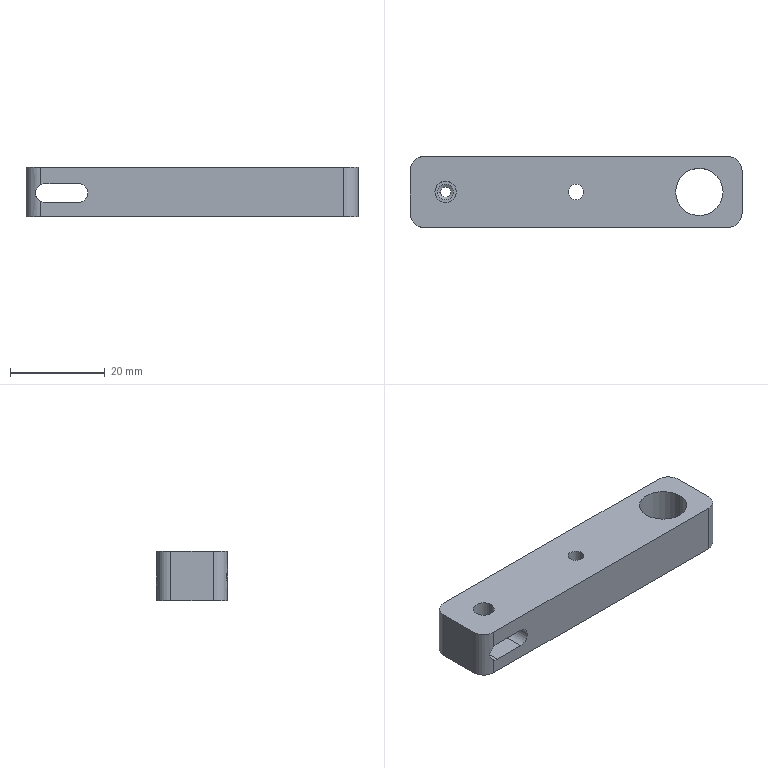Part | STEP file | 11-FG-B03911 | 1 solid | 24 faces | box 70 x 15 x 10.45 mm | volume 9294 mm3 | cylinder 14 | plane 8 | cone 2 | commonest cylinder face diameters 3.3 x4 6 x4 4 x2 4.5 x2 10 x2
STEP:
#1=CARTESIAN_POINT('',(-29.75,0.,7.));
#2=VERTEX_POINT('',#1);
#3=CARTESIAN_POINT('',(-25.25,0.,7.));
#4=VERTEX_POINT('',#3);
#5=CARTESIAN_POINT('',(-27.5,0.,7.));
#6=DIRECTION('',(0.,0.,1.));
#7=DIRECTION('',(1.,0.,0.));
#8=AXIS2_PLACEMENT_3D('',#5,#6,#7);
#9=CIRCLE('',#8,2.25);
#10=EDGE_CURVE('',#2,#4,#9,.T.);
#11=ORIENTED_EDGE('',*,*,#10,.F.);
#12=CARTESIAN_POINT('',(-29.75,0.,10.45));
#13=VERTEX_POINT('',#12);
#14=CARTESIAN_POINT('',(-29.75,0.,5.45));
#15=DIRECTION('',(0.,0.,1.));
#16=VECTOR('',#15,1000.);
#17=LINE('',#14,#16);
#18=EDGE_CURVE('',#2,#13,#17,.T.);
#19=ORIENTED_EDGE('',*,*,#18,.T.);
#20=CARTESIAN_POINT('',(-25.25,0.,10.45));
#21=VERTEX_POINT('',#20);
#22=CARTESIAN_POINT('',(-27.5,0.,10.45));
#23=DIRECTION('',(0.,0.,1.));
#24=DIRECTION('',(1.,0.,0.));
#25=AXIS2_PLACEMENT_3D('',#22,#23,#24);
#26=CIRCLE('',#25,2.25);
#27=EDGE_CURVE('',#13,#21,#26,.T.);
#28=ORIENTED_EDGE('',*,*,#27,.T.);
#29=CARTESIAN_POINT('',(-25.25,0.,5.45));
#30=DIRECTION('',(0.,0.,1.));
#31=VECTOR('',#30,1000.);
#32=LINE('',#29,#31);
#33=EDGE_CURVE('',#4,#21,#32,.T.);
#34=ORIENTED_EDGE('',*,*,#33,.F.);
#35=EDGE_LOOP('',(#11,#19,#28,#34));
#36=FACE_OUTER_BOUND('',#35,.T.);
#37=CARTESIAN_POINT('',(-27.5,0.,5.45));
#38=DIRECTION('',(0.,0.,1.));
#39=DIRECTION('',(1.,0.,0.));
#40=AXIS2_PLACEMENT_3D('',#37,#38,#39);
#41=CYLINDRICAL_SURFACE('',#40,2.25);
#42=ADVANCED_FACE('',(#36),#41,.F.);
#43=CARTESIAN_POINT('',(-1.65,0.,0.));
#44=VERTEX_POINT('',#43);
#45=CARTESIAN_POINT('',(1.65,0.,0.));
#46=VERTEX_POINT('',#45);
#47=CARTESIAN_POINT('',(0.,0.,0.));
#48=DIRECTION('',(0.,0.,1.));
#49=DIRECTION('',(1.,0.,0.));
#50=AXIS2_PLACEMENT_3D('',#47,#48,#49);
#51=CIRCLE('',#50,1.65);
#52=EDGE_CURVE('',#44,#46,#51,.T.);
#53=ORIENTED_EDGE('',*,*,#52,.F.);
#54=CARTESIAN_POINT('',(-1.65,0.,10.45));
#55=VERTEX_POINT('',#54);
#56=CARTESIAN_POINT('',(-1.65,0.,10.45));
#57=DIRECTION('',(0.,0.,1.));
#58=VECTOR('',#57,1000.);
#59=LINE('',#56,#58);
#60=EDGE_CURVE('',#44,#55,#59,.T.);
#61=ORIENTED_EDGE('',*,*,#60,.T.);
#62=CARTESIAN_POINT('',(1.65,0.,10.45));
#63=VERTEX_POINT('',#62);
#64=CARTESIAN_POINT('',(0.,0.,10.45));
#65=DIRECTION('',(0.,0.,1.));
#66=DIRECTION('',(1.,0.,0.));
#67=AXIS2_PLACEMENT_3D('',#64,#65,#66);
#68=CIRCLE('',#67,1.65);
#69=EDGE_CURVE('',#55,#63,#68,.T.);
#70=ORIENTED_EDGE('',*,*,#69,.T.);
#71=CARTESIAN_POINT('',(1.65,0.,10.45));
#72=DIRECTION('',(0.,0.,1.));
#73=VECTOR('',#72,1000.);
#74=LINE('',#71,#73);
#75=EDGE_CURVE('',#46,#63,#74,.T.);
#76=ORIENTED_EDGE('',*,*,#75,.F.);
#77=EDGE_LOOP('',(#53,#61,#70,#76));
#78=FACE_OUTER_BOUND('',#77,.T.);
#79=CARTESIAN_POINT('',(0.,0.,10.45));
#80=DIRECTION('',(0.,0.,1.));
#81=DIRECTION('',(1.,0.,0.));
#82=AXIS2_PLACEMENT_3D('',#79,#80,#81);
#83=CYLINDRICAL_SURFACE('',#82,1.65);
#84=ADVANCED_FACE('',(#78),#83,.F.);
#85=CARTESIAN_POINT('',(-29.15,0.,0.35));
#86=VERTEX_POINT('',#85);
#87=CARTESIAN_POINT('',(-25.85,0.,0.35));
#88=VERTEX_POINT('',#87);
#89=CARTESIAN_POINT('',(-27.5,0.,0.35));
#90=DIRECTION('',(0.,0.,1.));
#91=DIRECTION('',(1.,0.,0.));
#92=AXIS2_PLACEMENT_3D('',#89,#90,#91);
#93=CIRCLE('',#92,1.65);
#94=EDGE_CURVE('',#86,#88,#93,.T.);
#95=ORIENTED_EDGE('',*,*,#94,.F.);
#96=CARTESIAN_POINT('',(-29.15,0.,3.));
#97=VERTEX_POINT('',#96);
#98=CARTESIAN_POINT('',(-29.15,0.,10.45));
#99=DIRECTION('',(0.,0.,1.));
#100=VECTOR('',#99,1000.);
#101=LINE('',#98,#100);
#102=EDGE_CURVE('',#86,#97,#101,.T.);
#103=ORIENTED_EDGE('',*,*,#102,.T.);
#104=CARTESIAN_POINT('',(-25.85,0.,3.));
#105=VERTEX_POINT('',#104);
#106=CARTESIAN_POINT('',(-27.5,0.,3.));
#107=DIRECTION('',(0.,0.,1.));
#108=DIRECTION('',(-1.,0.,0.));
#109=AXIS2_PLACEMENT_3D('',#106,#107,#108);
#110=CIRCLE('',#109,1.65);
#111=EDGE_CURVE('',#97,#105,#110,.T.);
#112=ORIENTED_EDGE('',*,*,#111,.T.);
#113=CARTESIAN_POINT('',(-25.85,0.,10.45));
#114=DIRECTION('',(0.,0.,1.));
#115=VECTOR('',#114,1000.);
#116=LINE('',#113,#115);
#117=EDGE_CURVE('',#88,#105,#116,.T.);
#118=ORIENTED_EDGE('',*,*,#117,.F.);
#119=EDGE_LOOP('',(#95,#103,#112,#118));
#120=FACE_OUTER_BOUND('',#119,.T.);
#121=CARTESIAN_POINT('',(-27.5,0.,10.45));
#122=DIRECTION('',(0.,0.,1.));
#123=DIRECTION('',(1.,0.,0.));
#124=AXIS2_PLACEMENT_3D('',#121,#122,#123);
#125=CYLINDRICAL_SURFACE('',#124,1.65);
#126=ADVANCED_FACE('',(#120),#125,.F.);
#127=CARTESIAN_POINT('',(-28.568,0.,0.));
#128=VERTEX_POINT('',#127);
#129=CARTESIAN_POINT('',(-26.432,0.,0.));
#130=VERTEX_POINT('',#129);
#131=CARTESIAN_POINT('',(-27.5,0.,0.));
#132=DIRECTION('',(0.,0.,1.));
#133=DIRECTION('',(1.,0.,0.));
#134=AXIS2_PLACEMENT_3D('',#131,#132,#133);
#135=CIRCLE('',#134,1.068);
#136=EDGE_CURVE('',#128,#130,#135,.T.);
#137=ORIENTED_EDGE('',*,*,#136,.F.);
#138=CARTESIAN_POINT('',(-29.15,0.,0.35));
#139=DIRECTION('',(-0.8572,0.,0.515));
#140=VECTOR('',#139,1000.);
#141=LINE('',#138,#140);
#142=EDGE_CURVE('',#128,#86,#141,.T.);
#143=ORIENTED_EDGE('',*,*,#142,.T.);
#144=ORIENTED_EDGE('',*,*,#94,.T.);
#145=CARTESIAN_POINT('',(-25.85,0.,0.35));
#146=DIRECTION('',(0.8572,0.,0.515));
#147=VECTOR('',#146,1000.);
#148=LINE('',#145,#147);
#149=EDGE_CURVE('',#130,#88,#148,.T.);
#150=ORIENTED_EDGE('',*,*,#149,.F.);
#151=EDGE_LOOP('',(#137,#143,#144,#150));
#152=FACE_OUTER_BOUND('',#151,.T.);
#153=CARTESIAN_POINT('',(-27.5,0.,0.35));
#154=DIRECTION('',(0.,0.,1.));
#155=DIRECTION('',(1.,0.,0.));
#156=AXIS2_PLACEMENT_3D('',#153,#154,#155);
#157=CONICAL_SURFACE('',#156,1.65,1.03);
#158=ADVANCED_FACE('',(#152),#157,.F.);
#159=CARTESIAN_POINT('',(21.,0.,10.45));
#160=VERTEX_POINT('',#159);
#161=CARTESIAN_POINT('',(31.,0.,10.45));
#162=VERTEX_POINT('',#161);
#163=CARTESIAN_POINT('',(26.,0.,10.45));
#164=DIRECTION('',(0.,0.,1.));
#165=DIRECTION('',(1.,0.,0.));
#166=AXIS2_PLACEMENT_3D('',#163,#164,#165);
#167=CIRCLE('',#166,5.);
#168=EDGE_CURVE('',#160,#162,#167,.T.);
#169=ORIENTED_EDGE('',*,*,#168,.T.);
#170=CARTESIAN_POINT('',(31.,0.,0.));
#171=VERTEX_POINT('',#170);
#172=CARTESIAN_POINT('',(31.,0.,15.));
#173=DIRECTION('',(0.,0.,-1.));
#174=VECTOR('',#173,1000.);
#175=LINE('',#172,#174);
#176=EDGE_CURVE('',#162,#171,#175,.T.);
#177=ORIENTED_EDGE('',*,*,#176,.T.);
#178=CARTESIAN_POINT('',(21.,0.,0.));
#179=VERTEX_POINT('',#178);
#180=CARTESIAN_POINT('',(26.,0.,0.));
#181=DIRECTION('',(0.,0.,-1.));
#182=DIRECTION('',(-1.,0.,0.));
#183=AXIS2_PLACEMENT_3D('',#180,#181,#182);
#184=CIRCLE('',#183,5.);
#185=EDGE_CURVE('',#171,#179,#184,.T.);
#186=ORIENTED_EDGE('',*,*,#185,.T.);
#187=CARTESIAN_POINT('',(21.,0.,15.));
#188=DIRECTION('',(0.,0.,-1.));
#189=VECTOR('',#188,1000.);
#190=LINE('',#187,#189);
#191=EDGE_CURVE('',#160,#179,#190,.T.);
#192=ORIENTED_EDGE('',*,*,#191,.F.);
#193=EDGE_LOOP('',(#169,#177,#186,#192));
#194=FACE_OUTER_BOUND('',#193,.T.);
#195=CARTESIAN_POINT('',(26.,0.,15.));
#196=DIRECTION('',(0.,0.,-1.));
#197=DIRECTION('',(-1.,0.,0.));
#198=AXIS2_PLACEMENT_3D('',#195,#196,#197);
#199=CYLINDRICAL_SURFACE('',#198,5.);
#200=ADVANCED_FACE('',(#194),#199,.F.);
#201=CARTESIAN_POINT('',(35.,-4.5,10.45));
#202=VERTEX_POINT('',#201);
#203=CARTESIAN_POINT('',(35.,4.5,10.45));
#204=VERTEX_POINT('',#203);
#205=CARTESIAN_POINT('',(35.,7.5,10.45));
#206=DIRECTION('',(0.,1.,0.));
#207=VECTOR('',#206,1000.);
#208=LINE('',#205,#207);
#209=EDGE_CURVE('',#202,#204,#208,.T.);
#210=ORIENTED_EDGE('',*,*,#209,.F.);
#211=CARTESIAN_POINT('',(35.,-4.5,0.));
#212=VERTEX_POINT('',#211);
#213=CARTESIAN_POINT('',(35.,-4.5,10.45));
#214=DIRECTION('',(0.,0.,-1.));
#215=VECTOR('',#214,1000.);
#216=LINE('',#213,#215);
#217=EDGE_CURVE('',#202,#212,#216,.T.);
#218=ORIENTED_EDGE('',*,*,#217,.T.);
#219=CARTESIAN_POINT('',(35.,4.5,0.));
#220=VERTEX_POINT('',#219);
#221=CARTESIAN_POINT('',(35.,7.5,0.));
#222=DIRECTION('',(0.,1.,0.));
#223=VECTOR('',#222,1000.);
#224=LINE('',#221,#223);
#225=EDGE_CURVE('',#212,#220,#224,.T.);
#226=ORIENTED_EDGE('',*,*,#225,.T.);
#227=CARTESIAN_POINT('',(35.,4.5,10.45));
#228=DIRECTION('',(0.,0.,1.));
#229=VECTOR('',#228,1000.);
#230=LINE('',#227,#229);
#231=EDGE_CURVE('',#220,#204,#230,.T.);
#232=ORIENTED_EDGE('',*,*,#231,.T.);
#233=EDGE_LOOP('',(#210,#218,#226,#232));
#234=FACE_OUTER_BOUND('',#233,.T.);
#235=CARTESIAN_POINT('',(35.,7.5,10.45));
#236=DIRECTION('',(-1.,0.,0.));
#237=DIRECTION('',(0.,0.,1.));
#238=AXIS2_PLACEMENT_3D('',#235,#236,#237);
#239=PLANE('',#238);
#240=ADVANCED_FACE('',(#234),#239,.F.);
#241=CARTESIAN_POINT('',(-31.,7.5,7.));
#242=VERTEX_POINT('',#241);
#243=CARTESIAN_POINT('',(-24.,7.5,7.));
#244=VERTEX_POINT('',#243);
#245=CARTESIAN_POINT('',(-24.,7.5,7.));
#246=DIRECTION('',(1.,0.,0.));
#247=VECTOR('',#246,1000.);
#248=LINE('',#245,#247);
#249=EDGE_CURVE('',#242,#244,#248,.T.);
#250=ORIENTED_EDGE('',*,*,#249,.F.);
#251=CARTESIAN_POINT('',(-32.,7.5,6.732));
#252=VERTEX_POINT('',#251);
#253=CARTESIAN_POINT('',(-31.,7.5,5.));
#254=DIRECTION('',(0.,1.,0.));
#255=DIRECTION('',(0.,0.,1.));
#256=AXIS2_PLACEMENT_3D('',#253,#254,#255);
#257=CIRCLE('',#256,2.);
#258=EDGE_CURVE('',#252,#242,#257,.T.);
#259=ORIENTED_EDGE('',*,*,#258,.F.);
#260=CARTESIAN_POINT('',(-32.,7.5,10.45));
#261=VERTEX_POINT('',#260);
#262=CARTESIAN_POINT('',(-32.,7.5,10.45));
#263=DIRECTION('',(0.,0.,1.));
#264=VECTOR('',#263,1000.);
#265=LINE('',#262,#264);
#266=EDGE_CURVE('',#252,#261,#265,.T.);
#267=ORIENTED_EDGE('',*,*,#266,.T.);
#268=CARTESIAN_POINT('',(32.,7.5,10.45));
#269=VERTEX_POINT('',#268);
#270=CARTESIAN_POINT('',(-35.,7.5,10.45));
#271=DIRECTION('',(-1.,0.,0.));
#272=VECTOR('',#271,1000.);
#273=LINE('',#270,#272);
#274=EDGE_CURVE('',#269,#261,#273,.T.);
#275=ORIENTED_EDGE('',*,*,#274,.F.);
#276=CARTESIAN_POINT('',(32.,7.5,0.));
#277=VERTEX_POINT('',#276);
#278=CARTESIAN_POINT('',(32.,7.5,10.45));
#279=DIRECTION('',(0.,0.,-1.));
#280=VECTOR('',#279,1000.);
#281=LINE('',#278,#280);
#282=EDGE_CURVE('',#269,#277,#281,.T.);
#283=ORIENTED_EDGE('',*,*,#282,.T.);
#284=CARTESIAN_POINT('',(-32.,7.5,0.));
#285=VERTEX_POINT('',#284);
#286=CARTESIAN_POINT('',(-35.,7.5,0.));
#287=DIRECTION('',(-1.,0.,0.));
#288=VECTOR('',#287,1000.);
#289=LINE('',#286,#288);
#290=EDGE_CURVE('',#277,#285,#289,.T.);
#291=ORIENTED_EDGE('',*,*,#290,.T.);
#292=CARTESIAN_POINT('',(-32.,7.5,3.268));
#293=VERTEX_POINT('',#292);
#294=CARTESIAN_POINT('',(-32.,7.5,10.45));
#295=DIRECTION('',(0.,0.,1.));
#296=VECTOR('',#295,1000.);
#297=LINE('',#294,#296);
#298=EDGE_CURVE('',#285,#293,#297,.T.);
#299=ORIENTED_EDGE('',*,*,#298,.T.);
#300=CARTESIAN_POINT('',(-31.,7.5,3.));
#301=VERTEX_POINT('',#300);
#302=CARTESIAN_POINT('',(-31.,7.5,5.));
#303=DIRECTION('',(0.,1.,0.));
#304=DIRECTION('',(0.,0.,1.));
#305=AXIS2_PLACEMENT_3D('',#302,#303,#304);
#306=CIRCLE('',#305,2.);
#307=EDGE_CURVE('',#301,#293,#306,.T.);
#308=ORIENTED_EDGE('',*,*,#307,.F.);
#309=CARTESIAN_POINT('',(-24.,7.5,3.));
#310=VERTEX_POINT('',#309);
#311=CARTESIAN_POINT('',(-24.,7.5,3.));
#312=DIRECTION('',(-1.,0.,0.));
#313=VECTOR('',#312,1000.);
#314=LINE('',#311,#313);
#315=EDGE_CURVE('',#310,#301,#314,.T.);
#316=ORIENTED_EDGE('',*,*,#315,.F.);
#317=CARTESIAN_POINT('',(-24.,7.5,5.));
#318=DIRECTION('',(0.,1.,0.));
#319=DIRECTION('',(0.,0.,1.));
#320=AXIS2_PLACEMENT_3D('',#317,#318,#319);
#321=CIRCLE('',#320,2.);
#322=EDGE_CURVE('',#244,#310,#321,.T.);
#323=ORIENTED_EDGE('',*,*,#322,.F.);
#324=EDGE_LOOP('',(#250,#259,#267,#275,#283,#291,#299,#308,#316,#323));
#325=FACE_OUTER_BOUND('',#324,.T.);
#326=CARTESIAN_POINT('',(-35.,7.5,10.45));
#327=DIRECTION('',(0.,-1.,0.));
#328=DIRECTION('',(0.,0.,-1.));
#329=AXIS2_PLACEMENT_3D('',#326,#327,#328);
#330=PLANE('',#329);
#331=ADVANCED_FACE('',(#325),#330,.F.);
#332=CARTESIAN_POINT('',(-35.,4.5,0.));
#333=VERTEX_POINT('',#332);
#334=CARTESIAN_POINT('',(-35.,-4.5,0.));
#335=VERTEX_POINT('',#334);
#336=CARTESIAN_POINT('',(-35.,7.5,0.));
#337=DIRECTION('',(0.,-1.,0.));
#338=VECTOR('',#337,1000.);
#339=LINE('',#336,#338);
#340=EDGE_CURVE('',#333,#335,#339,.T.);
#341=ORIENTED_EDGE('',*,*,#340,.T.);
#342=CARTESIAN_POINT('',(-35.,-4.5,10.45));
#343=VERTEX_POINT('',#342);
#344=CARTESIAN_POINT('',(-35.,-4.5,10.45));
#345=DIRECTION('',(0.,0.,1.));
#346=VECTOR('',#345,1000.);
#347=LINE('',#344,#346);
#348=EDGE_CURVE('',#335,#343,#347,.T.);
#349=ORIENTED_EDGE('',*,*,#348,.T.);
#350=CARTESIAN_POINT('',(-35.,4.5,10.45));
#351=VERTEX_POINT('',#350);
#352=CARTESIAN_POINT('',(-35.,7.5,10.45));
#353=DIRECTION('',(0.,-1.,0.));
#354=VECTOR('',#353,1000.);
#355=LINE('',#352,#354);
#356=EDGE_CURVE('',#351,#343,#355,.T.);
#357=ORIENTED_EDGE('',*,*,#356,.F.);
#358=CARTESIAN_POINT('',(-35.,4.5,10.45));
#359=DIRECTION('',(0.,0.,-1.));
#360=VECTOR('',#359,1000.);
#361=LINE('',#358,#360);
#362=EDGE_CURVE('',#351,#333,#361,.T.);
#363=ORIENTED_EDGE('',*,*,#362,.T.);
#364=EDGE_LOOP('',(#341,#349,#357,#363));
#365=FACE_OUTER_BOUND('',#364,.T.);
#366=CARTESIAN_POINT('',(-35.,7.5,10.45));
#367=DIRECTION('',(1.,0.,0.));
#368=DIRECTION('',(0.,0.,-1.));
#369=AXIS2_PLACEMENT_3D('',#366,#367,#368);
#370=PLANE('',#369);
#371=ADVANCED_FACE('',(#365),#370,.F.);
#372=CARTESIAN_POINT('',(-32.,-7.5,10.45));
#373=VERTEX_POINT('',#372);
#374=CARTESIAN_POINT('',(-32.,-7.5,6.732));
#375=VERTEX_POINT('',#374);
#376=CARTESIAN_POINT('',(-32.,-7.5,10.45));
#377=DIRECTION('',(0.,0.,-1.));
#378=VECTOR('',#377,1000.);
#379=LINE('',#376,#378);
#380=EDGE_CURVE('',#373,#375,#379,.T.);
#381=ORIENTED_EDGE('',*,*,#380,.T.);
#382=CARTESIAN_POINT('',(-31.,-7.5,7.));
#383=VERTEX_POINT('',#382);
#384=CARTESIAN_POINT('',(-31.,-7.5,5.));
#385=DIRECTION('',(0.,1.,0.));
#386=DIRECTION('',(0.,0.,1.));
#387=AXIS2_PLACEMENT_3D('',#384,#385,#386);
#388=CIRCLE('',#387,2.);
#389=EDGE_CURVE('',#375,#383,#388,.T.);
#390=ORIENTED_EDGE('',*,*,#389,.T.);
#391=CARTESIAN_POINT('',(-24.,-7.5,7.));
#392=VERTEX_POINT('',#391);
#393=CARTESIAN_POINT('',(-24.,-7.5,7.));
#394=DIRECTION('',(1.,0.,0.));
#395=VECTOR('',#394,1000.);
#396=LINE('',#393,#395);
#397=EDGE_CURVE('',#383,#392,#396,.T.);
#398=ORIENTED_EDGE('',*,*,#397,.T.);
#399=CARTESIAN_POINT('',(-24.,-7.5,3.));
#400=VERTEX_POINT('',#399);
#401=CARTESIAN_POINT('',(-24.,-7.5,5.));
#402=DIRECTION('',(0.,1.,0.));
#403=DIRECTION('',(0.,0.,1.));
#404=AXIS2_PLACEMENT_3D('',#401,#402,#403);
#405=CIRCLE('',#404,2.);
#406=EDGE_CURVE('',#392,#400,#405,.T.);
#407=ORIENTED_EDGE('',*,*,#406,.T.);
#408=CARTESIAN_POINT('',(-31.,-7.5,3.));
#409=VERTEX_POINT('',#408);
#410=CARTESIAN_POINT('',(-24.,-7.5,3.));
#411=DIRECTION('',(-1.,0.,0.));
#412=VECTOR('',#411,1000.);
#413=LINE('',#410,#412);
#414=EDGE_CURVE('',#400,#409,#413,.T.);
#415=ORIENTED_EDGE('',*,*,#414,.T.);
#416=CARTESIAN_POINT('',(-32.,-7.5,3.268));
#417=VERTEX_POINT('',#416);
#418=CARTESIAN_POINT('',(-31.,-7.5,5.));
#419=DIRECTION('',(0.,1.,0.));
#420=DIRECTION('',(0.,0.,1.));
#421=AXIS2_PLACEMENT_3D('',#418,#419,#420);
#422=CIRCLE('',#421,2.);
#423=EDGE_CURVE('',#409,#417,#422,.T.);
#424=ORIENTED_EDGE('',*,*,#423,.T.);
#425=CARTESIAN_POINT('',(-32.,-7.5,0.));
#426=VERTEX_POINT('',#425);
#427=CARTESIAN_POINT('',(-32.,-7.5,10.45));
#428=DIRECTION('',(0.,0.,-1.));
#429=VECTOR('',#428,1000.);
#430=LINE('',#427,#429);
#431=EDGE_CURVE('',#417,#426,#430,.T.);
#432=ORIENTED_EDGE('',*,*,#431,.T.);
#433=CARTESIAN_POINT('',(32.,-7.5,0.));
#434=VERTEX_POINT('',#433);
#435=CARTESIAN_POINT('',(-35.,-7.5,0.));
#436=DIRECTION('',(1.,0.,0.));
#437=VECTOR('',#436,1000.);
#438=LINE('',#435,#437);
#439=EDGE_CURVE('',#426,#434,#438,.T.);
#440=ORIENTED_EDGE('',*,*,#439,.T.);
#441=CARTESIAN_POINT('',(32.,-7.5,10.45));
#442=VERTEX_POINT('',#441);
#443=CARTESIAN_POINT('',(32.,-7.5,10.45));
#444=DIRECTION('',(0.,0.,1.));
#445=VECTOR('',#444,1000.);
#446=LINE('',#443,#445);
#447=EDGE_CURVE('',#434,#442,#446,.T.);
#448=ORIENTED_EDGE('',*,*,#447,.T.);
#449=CARTESIAN_POINT('',(-35.,-7.5,10.45));
#450=DIRECTION('',(1.,0.,0.));
#451=VECTOR('',#450,1000.);
#452=LINE('',#449,#451);
#453=EDGE_CURVE('',#373,#442,#452,.T.);
#454=ORIENTED_EDGE('',*,*,#453,.F.);
#455=EDGE_LOOP('',(#381,#390,#398,#407,#415,#424,#432,#440,#448,#454));
#456=FACE_OUTER_BOUND('',#455,.T.);
#457=CARTESIAN_POINT('',(-35.,-7.5,10.45));
#458=DIRECTION('',(0.,1.,0.));
#459=DIRECTION('',(0.,0.,1.));
#460=AXIS2_PLACEMENT_3D('',#457,#458,#459);
#461=PLANE('',#460);
#462=ADVANCED_FACE('',(#456),#461,.F.);
#463=CARTESIAN_POINT('',(-27.5,0.,10.45));
#464=DIRECTION('',(0.,0.,1.));
#465=DIRECTION('',(1.,0.,0.));
#466=AXIS2_PLACEMENT_3D('',#463,#464,#465);
#467=CIRCLE('',#466,2.25);
#468=EDGE_CURVE('',#21,#13,#467,.T.);
#469=ORIENTED_EDGE('',*,*,#468,.F.);
#470=ORIENTED_EDGE('',*,*,#27,.F.);
#471=EDGE_LOOP('',(#469,#470));
#472=FACE_BOUND('',#471,.T.);
#473=CARTESIAN_POINT('',(0.,0.,10.45));
#474=DIRECTION('',(0.,0.,1.));
#475=DIRECTION('',(1.,0.,0.));
#476=AXIS2_PLACEMENT_3D('',#473,#474,#475);
#477=CIRCLE('',#476,1.65);
#478=EDGE_CURVE('',#63,#55,#477,.T.);
#479=ORIENTED_EDGE('',*,*,#478,.F.);
#480=ORIENTED_EDGE('',*,*,#69,.F.);
#481=EDGE_LOOP('',(#479,#480));
#482=FACE_BOUND('',#481,.T.);
#483=ORIENTED_EDGE('',*,*,#168,.F.);
#484=CARTESIAN_POINT('',(26.,0.,10.45));
#485=DIRECTION('',(0.,0.,1.));
#486=DIRECTION('',(1.,0.,0.));
#487=AXIS2_PLACEMENT_3D('',#484,#485,#486);
#488=CIRCLE('',#487,5.);
#489=EDGE_CURVE('',#162,#160,#488,.T.);
#490=ORIENTED_EDGE('',*,*,#489,.F.);
#491=EDGE_LOOP('',(#483,#490));
#492=FACE_BOUND('',#491,.T.);
#493=ORIENTED_EDGE('',*,*,#356,.T.);
#494=CARTESIAN_POINT('',(-32.,-4.5,10.45));
#495=DIRECTION('',(0.,0.,1.));
#496=DIRECTION('',(1.,0.,0.));
#497=AXIS2_PLACEMENT_3D('',#494,#495,#496);
#498=CIRCLE('',#497,3.);
#499=EDGE_CURVE('',#343,#373,#498,.T.);
#500=ORIENTED_EDGE('',*,*,#499,.T.);
#501=ORIENTED_EDGE('',*,*,#453,.T.);
#502=CARTESIAN_POINT('',(32.,-4.5,10.45));
#503=DIRECTION('',(0.,0.,1.));
#504=DIRECTION('',(1.,0.,0.));
#505=AXIS2_PLACEMENT_3D('',#502,#503,#504);
#506=CIRCLE('',#505,3.);
#507=EDGE_CURVE('',#442,#202,#506,.T.);
#508=ORIENTED_EDGE('',*,*,#507,.T.);
#509=ORIENTED_EDGE('',*,*,#209,.T.);
#510=CARTESIAN_POINT('',(32.,4.5,10.45));
#511=DIRECTION('',(0.,0.,1.));
#512=DIRECTION('',(1.,0.,0.));
#513=AXIS2_PLACEMENT_3D('',#510,#511,#512);
#514=CIRCLE('',#513,3.);
#515=EDGE_CURVE('',#204,#269,#514,.T.);
#516=ORIENTED_EDGE('',*,*,#515,.T.);
#517=ORIENTED_EDGE('',*,*,#274,.T.);
#518=CARTESIAN_POINT('',(-32.,4.5,10.45));
#519=DIRECTION('',(0.,0.,1.));
#520=DIRECTION('',(1.,0.,0.));
#521=AXIS2_PLACEMENT_3D('',#518,#519,#520);
#522=CIRCLE('',#521,3.);
#523=EDGE_CURVE('',#261,#351,#522,.T.);
#524=ORIENTED_EDGE('',*,*,#523,.T.);
#525=EDGE_LOOP('',(#493,#500,#501,#508,#509,#516,#517,#524));
#526=FACE_OUTER_BOUND('',#525,.T.);
#527=CARTESIAN_POINT('',(0.,0.,10.45));
#528=DIRECTION('',(0.,0.,1.));
#529=DIRECTION('',(1.,0.,0.));
#530=AXIS2_PLACEMENT_3D('',#527,#528,#529);
#531=PLANE('',#530);
#532=ADVANCED_FACE('',(#472,#482,#492,#526),#531,.T.);
#533=CARTESIAN_POINT('',(0.,0.,0.));
#534=DIRECTION('',(0.,0.,1.));
#535=DIRECTION('',(1.,0.,0.));
#536=AXIS2_PLACEMENT_3D('',#533,#534,#535);
#537=CIRCLE('',#536,1.65);
#538=EDGE_CURVE('',#46,#44,#537,.T.);
#539=ORIENTED_EDGE('',*,*,#538,.T.);
#540=ORIENTED_EDGE('',*,*,#52,.T.);
#541=EDGE_LOOP('',(#539,#540));
#542=FACE_BOUND('',#541,.T.);
#543=CARTESIAN_POINT('',(-27.5,0.,0.));
#544=DIRECTION('',(0.,0.,1.));
#545=DIRECTION('',(1.,0.,0.));
#546=AXIS2_PLACEMENT_3D('',#543,#544,#545);
#547=CIRCLE('',#546,1.068);
#548=EDGE_CURVE('',#130,#128,#547,.T.);
#549=ORIENTED_EDGE('',*,*,#548,.T.);
#550=ORIENTED_EDGE('',*,*,#136,.T.);
#551=EDGE_LOOP('',(#549,#550));
#552=FACE_BOUND('',#551,.T.);
#553=CARTESIAN_POINT('',(26.,0.,0.));
#554=DIRECTION('',(0.,0.,-1.));
#555=DIRECTION('',(-1.,0.,0.));
#556=AXIS2_PLACEMENT_3D('',#553,#554,#555);
#557=CIRCLE('',#556,5.);
#558=EDGE_CURVE('',#179,#171,#557,.T.);
#559=ORIENTED_EDGE('',*,*,#558,.F.);
#560=ORIENTED_EDGE('',*,*,#185,.F.);
#561=EDGE_LOOP('',(#559,#560));
#562=FACE_BOUND('',#561,.T.);
#563=ORIENTED_EDGE('',*,*,#439,.F.);
#564=CARTESIAN_POINT('',(-32.,-4.5,0.));
#565=DIRECTION('',(0.,0.,-1.));
#566=DIRECTION('',(1.,0.,0.));
#567=AXIS2_PLACEMENT_3D('',#564,#565,#566);
#568=CIRCLE('',#567,3.);
#569=EDGE_CURVE('',#426,#335,#568,.T.);
#570=ORIENTED_EDGE('',*,*,#569,.T.);
#571=ORIENTED_EDGE('',*,*,#340,.F.);
#572=CARTESIAN_POINT('',(-32.,4.5,0.));
#573=DIRECTION('',(0.,0.,-1.));
#574=DIRECTION('',(1.,0.,0.));
#575=AXIS2_PLACEMENT_3D('',#572,#573,#574);
#576=CIRCLE('',#575,3.);
#577=EDGE_CURVE('',#333,#285,#576,.T.);
#578=ORIENTED_EDGE('',*,*,#577,.T.);
#579=ORIENTED_EDGE('',*,*,#290,.F.);
#580=CARTESIAN_POINT('',(32.,4.5,0.));
#581=DIRECTION('',(0.,0.,-1.));
#582=DIRECTION('',(1.,0.,0.));
#583=AXIS2_PLACEMENT_3D('',#580,#581,#582);
#584=CIRCLE('',#583,3.);
#585=EDGE_CURVE('',#277,#220,#584,.T.);
#586=ORIENTED_EDGE('',*,*,#585,.T.);
#587=ORIENTED_EDGE('',*,*,#225,.F.);
#588=CARTESIAN_POINT('',(32.,-4.5,0.));
#589=DIRECTION('',(0.,0.,-1.));
#590=DIRECTION('',(1.,0.,0.));
#591=AXIS2_PLACEMENT_3D('',#588,#589,#590);
#592=CIRCLE('',#591,3.);
#593=EDGE_CURVE('',#212,#434,#592,.T.);
#594=ORIENTED_EDGE('',*,*,#593,.T.);
#595=EDGE_LOOP('',(#563,#570,#571,#578,#579,#586,#587,#594));
#596=FACE_OUTER_BOUND('',#595,.T.);
#597=CARTESIAN_POINT('',(0.,0.,0.));
#598=DIRECTION('',(0.,0.,1.));
#599=DIRECTION('',(1.,0.,0.));
#600=AXIS2_PLACEMENT_3D('',#597,#598,#599);
#601=PLANE('',#600);
#602=ADVANCED_FACE('',(#542,#552,#562,#596),#601,.F.);
#603=ORIENTED_EDGE('',*,*,#176,.F.);
#604=ORIENTED_EDGE('',*,*,#489,.T.);
#605=ORIENTED_EDGE('',*,*,#191,.T.);
#606=ORIENTED_EDGE('',*,*,#558,.T.);
#607=EDGE_LOOP('',(#603,#604,#605,#606));
#608=FACE_OUTER_BOUND('',#607,.T.);
#609=CARTESIAN_POINT('',(26.,0.,15.));
#610=DIRECTION('',(0.,0.,-1.));
#611=DIRECTION('',(-1.,0.,0.));
#612=AXIS2_PLACEMENT_3D('',#609,#610,#611);
#613=CYLINDRICAL_SURFACE('',#612,5.);
#614=ADVANCED_FACE('',(#608),#613,.F.);
#615=CARTESIAN_POINT('',(-32.,-7.5,6.732));
#616=CARTESIAN_POINT('',(-32.153,-7.5,6.644));
#617=CARTESIAN_POINT('',(-32.291,-7.488,6.537));
#618=CARTESIAN_POINT('',(-32.538,-7.454,6.291));
#619=CARTESIAN_POINT('',(-32.645,-7.431,6.151));
#620=CARTESIAN_POINT('',(-32.818,-7.388,5.851));
#621=CARTESIAN_POINT('',(-32.886,-7.366,5.687));
#622=CARTESIAN_POINT('',(-32.976,-7.337,5.352));
#623=CARTESIAN_POINT('',(-33.,-7.328,5.176));
#624=CARTESIAN_POINT('',(-33.,-7.328,4.825));
#625=CARTESIAN_POINT('',(-32.977,-7.337,4.653));
#626=CARTESIAN_POINT('',(-32.886,-7.366,4.313));
#627=CARTESIAN_POINT('',(-32.82,-7.387,4.152));
#628=CARTESIAN_POINT('',(-32.559,-7.453,3.7));
#629=CARTESIAN_POINT('',(-32.306,-7.5,3.445));
#630=CARTESIAN_POINT('',(-32.,-7.5,3.268));
#631=B_SPLINE_CURVE_WITH_KNOTS('',3,(#615,#616,#617,#618,#619,#620,#621,#622,#623,#624,#625,#626,#627,#628,#629,#630),.UNSPECIFIED.,.F.,.F.,(4,2,2,2,2,2,2,4),(0.,0.0005228,0.001046,0.001568,0.002091,0.002614,0.003137,0.004182),.UNSPECIFIED.);
#632=EDGE_CURVE('',#375,#417,#631,.T.);
#633=ORIENTED_EDGE('',*,*,#632,.F.);
#634=ORIENTED_EDGE('',*,*,#380,.F.);
#635=ORIENTED_EDGE('',*,*,#499,.F.);
#636=ORIENTED_EDGE('',*,*,#348,.F.);
#637=ORIENTED_EDGE('',*,*,#569,.F.);
#638=ORIENTED_EDGE('',*,*,#431,.F.);
#639=EDGE_LOOP('',(#633,#634,#635,#636,#637,#638));
#640=FACE_OUTER_BOUND('',#639,.T.);
#641=CARTESIAN_POINT('',(-32.,-4.5,10.45));
#642=DIRECTION('',(0.,0.,-1.));
#643=DIRECTION('',(-1.,0.,0.));
#644=AXIS2_PLACEMENT_3D('',#641,#642,#643);
#645=CYLINDRICAL_SURFACE('',#644,3.);
#646=ADVANCED_FACE('',(#640),#645,.T.);
#647=CARTESIAN_POINT('',(-32.,7.5,3.268));
#648=CARTESIAN_POINT('',(-32.153,7.5,3.356));
#649=CARTESIAN_POINT('',(-32.291,7.488,3.463));
#650=CARTESIAN_POINT('',(-32.538,7.454,3.709));
#651=CARTESIAN_POINT('',(-32.645,7.431,3.849));
#652=CARTESIAN_POINT('',(-32.818,7.388,4.149));
#653=CARTESIAN_POINT('',(-32.886,7.366,4.313));
#654=CARTESIAN_POINT('',(-32.976,7.337,4.648));
#655=CARTESIAN_POINT('',(-33.,7.328,4.824));
#656=CARTESIAN_POINT('',(-33.,7.328,5.175));
#657=CARTESIAN_POINT('',(-32.977,7.337,5.347));
#658=CARTESIAN_POINT('',(-32.886,7.366,5.687));
#659=CARTESIAN_POINT('',(-32.82,7.387,5.848));
#660=CARTESIAN_POINT('',(-32.559,7.453,6.3));
#661=CARTESIAN_POINT('',(-32.306,7.5,6.555));
#662=CARTESIAN_POINT('',(-32.,7.5,6.732));
#663=B_SPLINE_CURVE_WITH_KNOTS('',3,(#647,#648,#649,#650,#651,#652,#653,#654,#655,#656,#657,#658,#659,#660,#661,#662),.UNSPECIFIED.,.F.,.F.,(4,2,2,2,2,2,2,4),(0.,0.0005228,0.001046,0.001568,0.002091,0.002614,0.003137,0.004182),.UNSPECIFIED.);
#664=EDGE_CURVE('',#293,#252,#663,.T.);
#665=ORIENTED_EDGE('',*,*,#664,.F.);
#666=ORIENTED_EDGE('',*,*,#298,.F.);
#667=ORIENTED_EDGE('',*,*,#577,.F.);
#668=ORIENTED_EDGE('',*,*,#362,.F.);
#669=ORIENTED_EDGE('',*,*,#523,.F.);
#670=ORIENTED_EDGE('',*,*,#266,.F.);
#671=EDGE_LOOP('',(#665,#666,#667,#668,#669,#670));
#672=FACE_OUTER_BOUND('',#671,.T.);
#673=CARTESIAN_POINT('',(-32.,4.5,10.45));
#674=DIRECTION('',(0.,0.,-1.));
#675=DIRECTION('',(-1.,0.,0.));
#676=AXIS2_PLACEMENT_3D('',#673,#674,#675);
#677=CYLINDRICAL_SURFACE('',#676,3.);
#678=ADVANCED_FACE('',(#672),#677,.T.);
#679=ORIENTED_EDGE('',*,*,#507,.F.);
#680=ORIENTED_EDGE('',*,*,#447,.F.);
#681=ORIENTED_EDGE('',*,*,#593,.F.);
#682=ORIENTED_EDGE('',*,*,#217,.F.);
#683=EDGE_LOOP('',(#679,#680,#681,#682));
#684=FACE_OUTER_BOUND('',#683,.T.);
#685=CARTESIAN_POINT('',(32.,-4.5,10.45));
#686=DIRECTION('',(0.,0.,-1.));
#687=DIRECTION('',(-1.,0.,0.));
#688=AXIS2_PLACEMENT_3D('',#685,#686,#687);
#689=CYLINDRICAL_SURFACE('',#688,3.);
#690=ADVANCED_FACE('',(#684),#689,.T.);
#691=ORIENTED_EDGE('',*,*,#515,.F.);
#692=ORIENTED_EDGE('',*,*,#231,.F.);
#693=ORIENTED_EDGE('',*,*,#585,.F.);
#694=ORIENTED_EDGE('',*,*,#282,.F.);
#695=EDGE_LOOP('',(#691,#692,#693,#694));
#696=FACE_OUTER_BOUND('',#695,.T.);
#697=CARTESIAN_POINT('',(32.,4.5,10.45));
#698=DIRECTION('',(0.,0.,-1.));
#699=DIRECTION('',(-1.,0.,0.));
#700=AXIS2_PLACEMENT_3D('',#697,#698,#699);
#701=CYLINDRICAL_SURFACE('',#700,3.);
#702=ADVANCED_FACE('',(#696),#701,.T.);
#703=ORIENTED_EDGE('',*,*,#142,.F.);
#704=ORIENTED_EDGE('',*,*,#548,.F.);
#705=ORIENTED_EDGE('',*,*,#149,.T.);
#706=CARTESIAN_POINT('',(-27.5,0.,0.35));
#707=DIRECTION('',(0.,0.,1.));
#708=DIRECTION('',(1.,0.,0.));
#709=AXIS2_PLACEMENT_3D('',#706,#707,#708);
#710=CIRCLE('',#709,1.65);
#711=EDGE_CURVE('',#88,#86,#710,.T.);
#712=ORIENTED_EDGE('',*,*,#711,.T.);
#713=EDGE_LOOP('',(#703,#704,#705,#712));
#714=FACE_OUTER_BOUND('',#713,.T.);
#715=CARTESIAN_POINT('',(-27.5,0.,0.35));
#716=DIRECTION('',(0.,0.,1.));
#717=DIRECTION('',(1.,0.,0.));
#718=AXIS2_PLACEMENT_3D('',#715,#716,#717);
#719=CONICAL_SURFACE('',#718,1.65,1.03);
#720=ADVANCED_FACE('',(#714),#719,.F.);
#721=ORIENTED_EDGE('',*,*,#102,.F.);
#722=ORIENTED_EDGE('',*,*,#711,.F.);
#723=ORIENTED_EDGE('',*,*,#117,.T.);
#724=CARTESIAN_POINT('',(-27.5,0.,3.));
#725=DIRECTION('',(0.,0.,1.));
#726=DIRECTION('',(-1.,0.,0.));
#727=AXIS2_PLACEMENT_3D('',#724,#725,#726);
#728=CIRCLE('',#727,1.65);
#729=EDGE_CURVE('',#105,#97,#728,.T.);
#730=ORIENTED_EDGE('',*,*,#729,.T.);
#731=EDGE_LOOP('',(#721,#722,#723,#730));
#732=FACE_OUTER_BOUND('',#731,.T.);
#733=CARTESIAN_POINT('',(-27.5,0.,10.45));
#734=DIRECTION('',(0.,0.,1.));
#735=DIRECTION('',(1.,0.,0.));
#736=AXIS2_PLACEMENT_3D('',#733,#734,#735);
#737=CYLINDRICAL_SURFACE('',#736,1.65);
#738=ADVANCED_FACE('',(#732),#737,.F.);
#739=CARTESIAN_POINT('',(-27.5,0.,7.));
#740=DIRECTION('',(0.,0.,1.));
#741=DIRECTION('',(1.,0.,0.));
#742=AXIS2_PLACEMENT_3D('',#739,#740,#741);
#743=CIRCLE('',#742,2.25);
#744=EDGE_CURVE('',#4,#2,#743,.T.);
#745=ORIENTED_EDGE('',*,*,#744,.T.);
#746=ORIENTED_EDGE('',*,*,#10,.T.);
#747=EDGE_LOOP('',(#745,#746));
#748=FACE_BOUND('',#747,.T.);
#749=ORIENTED_EDGE('',*,*,#249,.T.);
#750=CARTESIAN_POINT('',(-24.,-7.5,7.));
#751=DIRECTION('',(0.,1.,0.));
#752=VECTOR('',#751,1000.);
#753=LINE('',#750,#752);
#754=EDGE_CURVE('',#392,#244,#753,.T.);
#755=ORIENTED_EDGE('',*,*,#754,.F.);
#756=ORIENTED_EDGE('',*,*,#397,.F.);
#757=CARTESIAN_POINT('',(-31.,-7.5,7.));
#758=DIRECTION('',(0.,1.,0.));
#759=VECTOR('',#758,1000.);
#760=LINE('',#757,#759);
#761=EDGE_CURVE('',#383,#242,#760,.T.);
#762=ORIENTED_EDGE('',*,*,#761,.T.);
#763=EDGE_LOOP('',(#749,#755,#756,#762));
#764=FACE_OUTER_BOUND('',#763,.T.);
#765=CARTESIAN_POINT('',(-24.,-7.5,7.));
#766=DIRECTION('',(0.,0.,1.));
#767=DIRECTION('',(1.,0.,0.));
#768=AXIS2_PLACEMENT_3D('',#765,#766,#767);
#769=PLANE('',#768);
#770=ADVANCED_FACE('',(#748,#764),#769,.F.);
#771=ORIENTED_EDGE('',*,*,#315,.T.);
#772=CARTESIAN_POINT('',(-31.,-7.5,3.));
#773=DIRECTION('',(0.,1.,0.));
#774=VECTOR('',#773,1000.);
#775=LINE('',#772,#774);
#776=EDGE_CURVE('',#409,#301,#775,.T.);
#777=ORIENTED_EDGE('',*,*,#776,.F.);
#778=ORIENTED_EDGE('',*,*,#414,.F.);
#779=CARTESIAN_POINT('',(-24.,-7.5,3.));
#780=DIRECTION('',(0.,1.,0.));
#781=VECTOR('',#780,1000.);
#782=LINE('',#779,#781);
#783=EDGE_CURVE('',#400,#310,#782,.T.);
#784=ORIENTED_EDGE('',*,*,#783,.T.);
#785=EDGE_LOOP('',(#771,#777,#778,#784));
#786=FACE_OUTER_BOUND('',#785,.T.);
#787=ORIENTED_EDGE('',*,*,#729,.F.);
#788=ORIENTED_EDGE('',*,*,#111,.F.);
#789=EDGE_LOOP('',(#787,#788));
#790=FACE_BOUND('',#789,.T.);
#791=CARTESIAN_POINT('',(-24.,-7.5,3.));
#792=DIRECTION('',(0.,0.,-1.));
#793=DIRECTION('',(-1.,0.,0.));
#794=AXIS2_PLACEMENT_3D('',#791,#792,#793);
#795=PLANE('',#794);
#796=ADVANCED_FACE('',(#786,#790),#795,.F.);
#797=ORIENTED_EDGE('',*,*,#322,.T.);
#798=ORIENTED_EDGE('',*,*,#783,.F.);
#799=ORIENTED_EDGE('',*,*,#406,.F.);
#800=ORIENTED_EDGE('',*,*,#754,.T.);
#801=EDGE_LOOP('',(#797,#798,#799,#800));
#802=FACE_OUTER_BOUND('',#801,.T.);
#803=CARTESIAN_POINT('',(-24.,-7.5,5.));
#804=DIRECTION('',(0.,1.,0.));
#805=DIRECTION('',(0.,0.,1.));
#806=AXIS2_PLACEMENT_3D('',#803,#804,#805);
#807=CYLINDRICAL_SURFACE('',#806,2.);
#808=ADVANCED_FACE('',(#802),#807,.F.);
#809=ORIENTED_EDGE('',*,*,#632,.T.);
#810=ORIENTED_EDGE('',*,*,#423,.F.);
#811=ORIENTED_EDGE('',*,*,#776,.T.);
#812=ORIENTED_EDGE('',*,*,#307,.T.);
#813=ORIENTED_EDGE('',*,*,#664,.T.);
#814=ORIENTED_EDGE('',*,*,#258,.T.);
#815=ORIENTED_EDGE('',*,*,#761,.F.);
#816=ORIENTED_EDGE('',*,*,#389,.F.);
#817=EDGE_LOOP('',(#809,#810,#811,#812,#813,#814,#815,#816));
#818=FACE_OUTER_BOUND('',#817,.T.);
#819=CARTESIAN_POINT('',(-31.,-7.5,5.));
#820=DIRECTION('',(0.,1.,0.));
#821=DIRECTION('',(0.,0.,1.));
#822=AXIS2_PLACEMENT_3D('',#819,#820,#821);
#823=CYLINDRICAL_SURFACE('',#822,2.);
#824=ADVANCED_FACE('',(#818),#823,.F.);
#825=ORIENTED_EDGE('',*,*,#60,.F.);
#826=ORIENTED_EDGE('',*,*,#538,.F.);
#827=ORIENTED_EDGE('',*,*,#75,.T.);
#828=ORIENTED_EDGE('',*,*,#478,.T.);
#829=EDGE_LOOP('',(#825,#826,#827,#828));
#830=FACE_OUTER_BOUND('',#829,.T.);
#831=CARTESIAN_POINT('',(0.,0.,10.45));
#832=DIRECTION('',(0.,0.,1.));
#833=DIRECTION('',(1.,0.,0.));
#834=AXIS2_PLACEMENT_3D('',#831,#832,#833);
#835=CYLINDRICAL_SURFACE('',#834,1.65);
#836=ADVANCED_FACE('',(#830),#835,.F.);
#837=ORIENTED_EDGE('',*,*,#18,.F.);
#838=ORIENTED_EDGE('',*,*,#744,.F.);
#839=ORIENTED_EDGE('',*,*,#33,.T.);
#840=ORIENTED_EDGE('',*,*,#468,.T.);
#841=EDGE_LOOP('',(#837,#838,#839,#840));
#842=FACE_OUTER_BOUND('',#841,.T.);
#843=CARTESIAN_POINT('',(-27.5,0.,5.45));
#844=DIRECTION('',(0.,0.,1.));
#845=DIRECTION('',(1.,0.,0.));
#846=AXIS2_PLACEMENT_3D('',#843,#844,#845);
#847=CYLINDRICAL_SURFACE('',#846,2.25);
#848=ADVANCED_FACE('',(#842),#847,.F.);
#849=CLOSED_SHELL('',(#42,#84,#126,#158,#200,#240,#331,#371,#462,#532,#602,#614,#646,#678,#690,#702,#720,#738,#770,#796,#808,#824,#836,#848));
#850=MANIFOLD_SOLID_BREP('',#849);
#851=CARTESIAN_POINT('',(0.,0.,0.));
#852=DIRECTION('',(0.,0.,1.));
#853=DIRECTION('',(1.,0.,0.));
#854=AXIS2_PLACEMENT_3D('',#851,#852,#853);
#855=(LENGTH_UNIT()NAMED_UNIT(*)SI_UNIT(.MILLI.,.METRE.));
#856=UNCERTAINTY_MEASURE_WITH_UNIT(LENGTH_MEASURE(0.00001),#855,'','');
#857=(NAMED_UNIT(*)PLANE_ANGLE_UNIT()SI_UNIT($,.RADIAN.));
#858=(NAMED_UNIT(*)SI_UNIT($,.STERADIAN.)SOLID_ANGLE_UNIT());
#859=(GEOMETRIC_REPRESENTATION_CONTEXT(3)GLOBAL_UNCERTAINTY_ASSIGNED_CONTEXT((#856))GLOBAL_UNIT_ASSIGNED_CONTEXT((#855,#857,#858))REPRESENTATION_CONTEXT('',''));
#860=ADVANCED_BREP_SHAPE_REPRESENTATION('',(#850,#854),#859);